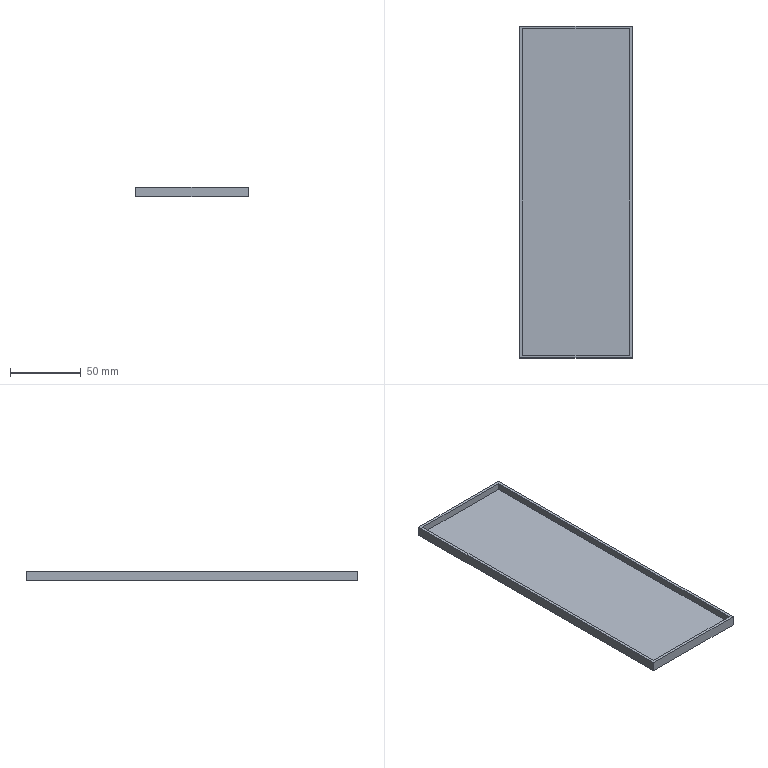Part | NX | features solid 2 | 1 solid | 11 faces | box 79.493 x 234.569 x 7 mm | volume 43494 mm3 | plane 11
STEP:
#1=CARTESIAN_POINT('',(-81.813,268.431,-296.));
#2=VERTEX_POINT('',#1);
#3=CARTESIAN_POINT('',(-161.306,268.431,-296.));
#4=VERTEX_POINT('',#3);
#5=CARTESIAN_POINT('',(-84.813,268.431,-296.));
#6=DIRECTION('',(-1.,0.,0.));
#7=VECTOR('',#6,1000.);
#8=LINE('',#5,#7);
#9=EDGE_CURVE('',#2,#4,#8,.T.);
#10=ORIENTED_EDGE('',*,*,#9,.T.);
#11=CARTESIAN_POINT('',(-161.306,268.431,-303.));
#12=VERTEX_POINT('',#11);
#13=CARTESIAN_POINT('',(-161.306,268.431,-303.));
#14=DIRECTION('',(0.,0.,1.));
#15=VECTOR('',#14,1000.);
#16=LINE('',#13,#15);
#17=EDGE_CURVE('',#12,#4,#16,.T.);
#18=ORIENTED_EDGE('',*,*,#17,.F.);
#19=CARTESIAN_POINT('',(-81.813,268.431,-303.));
#20=VERTEX_POINT('',#19);
#21=CARTESIAN_POINT('',(-84.813,268.431,-303.));
#22=DIRECTION('',(-1.,0.,0.));
#23=VECTOR('',#22,1000.);
#24=LINE('',#21,#23);
#25=EDGE_CURVE('',#20,#12,#24,.T.);
#26=ORIENTED_EDGE('',*,*,#25,.F.);
#27=CARTESIAN_POINT('',(-81.813,268.431,-303.));
#28=DIRECTION('',(0.,0.,1.));
#29=VECTOR('',#28,1000.);
#30=LINE('',#27,#29);
#31=EDGE_CURVE('',#20,#2,#30,.T.);
#32=ORIENTED_EDGE('',*,*,#31,.T.);
#33=EDGE_LOOP('',(#10,#18,#26,#32));
#34=FACE_BOUND('',#33,.T.);
#35=CARTESIAN_POINT('',(-84.813,268.431,-303.));
#36=DIRECTION('',(0.,1.,0.));
#37=DIRECTION('',(0.,0.,1.));
#38=AXIS2_PLACEMENT_3D('',#35,#36,#37);
#39=PLANE('',#38);
#40=ADVANCED_FACE('',(#34),#39,.F.);
#41=CARTESIAN_POINT('',(-161.306,503.,-296.));
#42=VERTEX_POINT('',#41);
#43=CARTESIAN_POINT('',(-161.306,311.431,-296.));
#44=DIRECTION('',(0.,1.,0.));
#45=VECTOR('',#44,1000.);
#46=LINE('',#43,#45);
#47=EDGE_CURVE('',#4,#42,#46,.T.);
#48=ORIENTED_EDGE('',*,*,#47,.T.);
#49=CARTESIAN_POINT('',(-161.306,503.,-303.));
#50=VERTEX_POINT('',#49);
#51=CARTESIAN_POINT('',(-161.306,503.,-303.));
#52=DIRECTION('',(0.,0.,1.));
#53=VECTOR('',#52,1000.);
#54=LINE('',#51,#53);
#55=EDGE_CURVE('',#50,#42,#54,.T.);
#56=ORIENTED_EDGE('',*,*,#55,.F.);
#57=CARTESIAN_POINT('',(-161.306,311.431,-303.));
#58=DIRECTION('',(0.,1.,0.));
#59=VECTOR('',#58,1000.);
#60=LINE('',#57,#59);
#61=EDGE_CURVE('',#12,#50,#60,.T.);
#62=ORIENTED_EDGE('',*,*,#61,.F.);
#63=ORIENTED_EDGE('',*,*,#17,.T.);
#64=EDGE_LOOP('',(#48,#56,#62,#63));
#65=FACE_BOUND('',#64,.T.);
#66=CARTESIAN_POINT('',(-161.306,311.431,-303.));
#67=DIRECTION('',(1.,0.,0.));
#68=DIRECTION('',(0.,0.,-1.));
#69=AXIS2_PLACEMENT_3D('',#66,#67,#68);
#70=PLANE('',#69);
#71=ADVANCED_FACE('',(#65),#70,.F.);
#72=CARTESIAN_POINT('',(-81.813,503.,-296.));
#73=VERTEX_POINT('',#72);
#74=CARTESIAN_POINT('',(-340.,503.,-296.));
#75=DIRECTION('',(1.,0.,0.));
#76=VECTOR('',#75,1000.);
#77=LINE('',#74,#76);
#78=EDGE_CURVE('',#42,#73,#77,.T.);
#79=ORIENTED_EDGE('',*,*,#78,.T.);
#80=CARTESIAN_POINT('',(-81.813,503.,-303.));
#81=VERTEX_POINT('',#80);
#82=CARTESIAN_POINT('',(-81.813,503.,-303.));
#83=DIRECTION('',(0.,0.,1.));
#84=VECTOR('',#83,1000.);
#85=LINE('',#82,#84);
#86=EDGE_CURVE('',#81,#73,#85,.T.);
#87=ORIENTED_EDGE('',*,*,#86,.F.);
#88=CARTESIAN_POINT('',(-340.,503.,-303.));
#89=DIRECTION('',(1.,0.,0.));
#90=VECTOR('',#89,1000.);
#91=LINE('',#88,#90);
#92=EDGE_CURVE('',#50,#81,#91,.T.);
#93=ORIENTED_EDGE('',*,*,#92,.F.);
#94=ORIENTED_EDGE('',*,*,#55,.T.);
#95=EDGE_LOOP('',(#79,#87,#93,#94));
#96=FACE_BOUND('',#95,.T.);
#97=CARTESIAN_POINT('',(-340.,503.,-303.));
#98=DIRECTION('',(0.,-1.,0.));
#99=DIRECTION('',(1.,0.,0.));
#100=AXIS2_PLACEMENT_3D('',#97,#98,#99);
#101=PLANE('',#100);
#102=ADVANCED_FACE('',(#96),#101,.F.);
#103=CARTESIAN_POINT('',(-81.813,500.89,-296.));
#104=DIRECTION('',(0.,-1.,0.));
#105=VECTOR('',#104,1000.);
#106=LINE('',#103,#105);
#107=EDGE_CURVE('',#73,#2,#106,.T.);
#108=ORIENTED_EDGE('',*,*,#107,.T.);
#109=ORIENTED_EDGE('',*,*,#31,.F.);
#110=CARTESIAN_POINT('',(-81.813,500.89,-303.));
#111=DIRECTION('',(0.,-1.,0.));
#112=VECTOR('',#111,1000.);
#113=LINE('',#110,#112);
#114=EDGE_CURVE('',#81,#20,#113,.T.);
#115=ORIENTED_EDGE('',*,*,#114,.F.);
#116=ORIENTED_EDGE('',*,*,#86,.T.);
#117=EDGE_LOOP('',(#108,#109,#115,#116));
#118=FACE_BOUND('',#117,.T.);
#119=CARTESIAN_POINT('',(-81.813,500.89,-303.));
#120=DIRECTION('',(-1.,0.,0.));
#121=DIRECTION('',(0.,0.,1.));
#122=AXIS2_PLACEMENT_3D('',#119,#120,#121);
#123=PLANE('',#122);
#124=ADVANCED_FACE('',(#118),#123,.F.);
#125=ORIENTED_EDGE('',*,*,#25,.T.);
#126=ORIENTED_EDGE('',*,*,#61,.T.);
#127=ORIENTED_EDGE('',*,*,#92,.T.);
#128=ORIENTED_EDGE('',*,*,#114,.T.);
#129=EDGE_LOOP('',(#125,#126,#127,#128));
#130=FACE_BOUND('',#129,.T.);
#131=CARTESIAN_POINT('',(-158.306,311.431,-303.));
#132=DIRECTION('',(0.,0.,-1.));
#133=DIRECTION('',(-1.,0.,0.));
#134=AXIS2_PLACEMENT_3D('',#131,#132,#133);
#135=PLANE('',#134);
#136=ADVANCED_FACE('',(#130),#135,.T.);
#137=CARTESIAN_POINT('',(-83.813,501.,-296.));
#138=VERTEX_POINT('',#137);
#139=CARTESIAN_POINT('',(-83.813,270.431,-296.));
#140=VERTEX_POINT('',#139);
#141=CARTESIAN_POINT('',(-83.813,500.89,-296.));
#142=DIRECTION('',(0.,-1.,0.));
#143=VECTOR('',#142,1000.);
#144=LINE('',#141,#143);
#145=EDGE_CURVE('',#138,#140,#144,.T.);
#146=ORIENTED_EDGE('',*,*,#145,.T.);
#147=CARTESIAN_POINT('',(-159.306,270.431,-296.));
#148=VERTEX_POINT('',#147);
#149=CARTESIAN_POINT('',(-84.813,270.431,-296.));
#150=DIRECTION('',(-1.,0.,0.));
#151=VECTOR('',#150,1000.);
#152=LINE('',#149,#151);
#153=EDGE_CURVE('',#140,#148,#152,.T.);
#154=ORIENTED_EDGE('',*,*,#153,.T.);
#155=CARTESIAN_POINT('',(-159.306,501.,-296.));
#156=VERTEX_POINT('',#155);
#157=CARTESIAN_POINT('',(-159.306,311.431,-296.));
#158=DIRECTION('',(0.,1.,0.));
#159=VECTOR('',#158,1000.);
#160=LINE('',#157,#159);
#161=EDGE_CURVE('',#148,#156,#160,.T.);
#162=ORIENTED_EDGE('',*,*,#161,.T.);
#163=CARTESIAN_POINT('',(-340.,501.,-296.));
#164=DIRECTION('',(1.,0.,0.));
#165=VECTOR('',#164,1000.);
#166=LINE('',#163,#165);
#167=EDGE_CURVE('',#156,#138,#166,.T.);
#168=ORIENTED_EDGE('',*,*,#167,.T.);
#169=EDGE_LOOP('',(#146,#154,#162,#168));
#170=FACE_BOUND('',#169,.T.);
#171=ORIENTED_EDGE('',*,*,#9,.F.);
#172=ORIENTED_EDGE('',*,*,#107,.F.);
#173=ORIENTED_EDGE('',*,*,#78,.F.);
#174=ORIENTED_EDGE('',*,*,#47,.F.);
#175=EDGE_LOOP('',(#171,#172,#173,#174));
#176=FACE_BOUND('',#175,.T.);
#177=CARTESIAN_POINT('',(-158.306,311.431,-296.));
#178=DIRECTION('',(0.,0.,-1.));
#179=DIRECTION('',(-1.,0.,0.));
#180=AXIS2_PLACEMENT_3D('',#177,#178,#179);
#181=PLANE('',#180);
#182=ADVANCED_FACE('',(#170,#176),#181,.F.);
#183=ORIENTED_EDGE('',*,*,#153,.F.);
#184=CARTESIAN_POINT('',(-83.813,270.431,-301.));
#185=VERTEX_POINT('',#184);
#186=CARTESIAN_POINT('',(-83.813,270.431,-303.));
#187=DIRECTION('',(0.,0.,1.));
#188=VECTOR('',#187,1000.);
#189=LINE('',#186,#188);
#190=EDGE_CURVE('',#185,#140,#189,.T.);
#191=ORIENTED_EDGE('',*,*,#190,.F.);
#192=CARTESIAN_POINT('',(-159.306,270.431,-301.));
#193=VERTEX_POINT('',#192);
#194=CARTESIAN_POINT('',(-84.813,270.431,-301.));
#195=DIRECTION('',(-1.,0.,0.));
#196=VECTOR('',#195,1000.);
#197=LINE('',#194,#196);
#198=EDGE_CURVE('',#185,#193,#197,.T.);
#199=ORIENTED_EDGE('',*,*,#198,.T.);
#200=CARTESIAN_POINT('',(-159.306,270.431,-303.));
#201=DIRECTION('',(0.,0.,1.));
#202=VECTOR('',#201,1000.);
#203=LINE('',#200,#202);
#204=EDGE_CURVE('',#193,#148,#203,.T.);
#205=ORIENTED_EDGE('',*,*,#204,.T.);
#206=EDGE_LOOP('',(#183,#191,#199,#205));
#207=FACE_BOUND('',#206,.T.);
#208=CARTESIAN_POINT('',(-84.813,270.431,-303.));
#209=DIRECTION('',(0.,1.,0.));
#210=DIRECTION('',(0.,0.,1.));
#211=AXIS2_PLACEMENT_3D('',#208,#209,#210);
#212=PLANE('',#211);
#213=ADVANCED_FACE('',(#207),#212,.T.);
#214=ORIENTED_EDGE('',*,*,#161,.F.);
#215=ORIENTED_EDGE('',*,*,#204,.F.);
#216=CARTESIAN_POINT('',(-159.306,501.,-301.));
#217=VERTEX_POINT('',#216);
#218=CARTESIAN_POINT('',(-159.306,311.431,-301.));
#219=DIRECTION('',(0.,1.,0.));
#220=VECTOR('',#219,1000.);
#221=LINE('',#218,#220);
#222=EDGE_CURVE('',#193,#217,#221,.T.);
#223=ORIENTED_EDGE('',*,*,#222,.T.);
#224=CARTESIAN_POINT('',(-159.306,501.,-303.));
#225=DIRECTION('',(0.,0.,1.));
#226=VECTOR('',#225,1000.);
#227=LINE('',#224,#226);
#228=EDGE_CURVE('',#217,#156,#227,.T.);
#229=ORIENTED_EDGE('',*,*,#228,.T.);
#230=EDGE_LOOP('',(#214,#215,#223,#229));
#231=FACE_BOUND('',#230,.T.);
#232=CARTESIAN_POINT('',(-159.306,311.431,-303.));
#233=DIRECTION('',(1.,0.,0.));
#234=DIRECTION('',(0.,0.,-1.));
#235=AXIS2_PLACEMENT_3D('',#232,#233,#234);
#236=PLANE('',#235);
#237=ADVANCED_FACE('',(#231),#236,.T.);
#238=ORIENTED_EDGE('',*,*,#167,.F.);
#239=ORIENTED_EDGE('',*,*,#228,.F.);
#240=CARTESIAN_POINT('',(-83.813,501.,-301.));
#241=VERTEX_POINT('',#240);
#242=CARTESIAN_POINT('',(-340.,501.,-301.));
#243=DIRECTION('',(1.,0.,0.));
#244=VECTOR('',#243,1000.);
#245=LINE('',#242,#244);
#246=EDGE_CURVE('',#217,#241,#245,.T.);
#247=ORIENTED_EDGE('',*,*,#246,.T.);
#248=CARTESIAN_POINT('',(-83.813,501.,-303.));
#249=DIRECTION('',(0.,0.,1.));
#250=VECTOR('',#249,1000.);
#251=LINE('',#248,#250);
#252=EDGE_CURVE('',#241,#138,#251,.T.);
#253=ORIENTED_EDGE('',*,*,#252,.T.);
#254=EDGE_LOOP('',(#238,#239,#247,#253));
#255=FACE_BOUND('',#254,.T.);
#256=CARTESIAN_POINT('',(-340.,501.,-303.));
#257=DIRECTION('',(0.,-1.,0.));
#258=DIRECTION('',(1.,0.,0.));
#259=AXIS2_PLACEMENT_3D('',#256,#257,#258);
#260=PLANE('',#259);
#261=ADVANCED_FACE('',(#255),#260,.T.);
#262=ORIENTED_EDGE('',*,*,#145,.F.);
#263=ORIENTED_EDGE('',*,*,#252,.F.);
#264=CARTESIAN_POINT('',(-83.813,500.89,-301.));
#265=DIRECTION('',(0.,-1.,0.));
#266=VECTOR('',#265,1000.);
#267=LINE('',#264,#266);
#268=EDGE_CURVE('',#241,#185,#267,.T.);
#269=ORIENTED_EDGE('',*,*,#268,.T.);
#270=ORIENTED_EDGE('',*,*,#190,.T.);
#271=EDGE_LOOP('',(#262,#263,#269,#270));
#272=FACE_BOUND('',#271,.T.);
#273=CARTESIAN_POINT('',(-83.813,500.89,-303.));
#274=DIRECTION('',(-1.,0.,0.));
#275=DIRECTION('',(0.,0.,1.));
#276=AXIS2_PLACEMENT_3D('',#273,#274,#275);
#277=PLANE('',#276);
#278=ADVANCED_FACE('',(#272),#277,.T.);
#279=ORIENTED_EDGE('',*,*,#198,.F.);
#280=ORIENTED_EDGE('',*,*,#268,.F.);
#281=ORIENTED_EDGE('',*,*,#246,.F.);
#282=ORIENTED_EDGE('',*,*,#222,.F.);
#283=EDGE_LOOP('',(#279,#280,#281,#282));
#284=FACE_BOUND('',#283,.T.);
#285=CARTESIAN_POINT('',(-158.306,311.431,-301.));
#286=DIRECTION('',(0.,0.,-1.));
#287=DIRECTION('',(-1.,0.,0.));
#288=AXIS2_PLACEMENT_3D('',#285,#286,#287);
#289=PLANE('',#288);
#290=ADVANCED_FACE('',(#284),#289,.F.);
#291=CLOSED_SHELL('',(#40,#71,#102,#124,#136,#182,#213,#237,#261,#278,#290));
#292=MANIFOLD_SOLID_BREP('',#291);
#293=(LENGTH_UNIT()NAMED_UNIT(*)SI_UNIT(.MILLI.,.METRE.));
#294=UNCERTAINTY_MEASURE_WITH_UNIT(LENGTH_MEASURE(0.00001),#293,'','');
#295=(NAMED_UNIT(*)PLANE_ANGLE_UNIT()SI_UNIT($,.RADIAN.));
#296=(NAMED_UNIT(*)SI_UNIT($,.STERADIAN.)SOLID_ANGLE_UNIT());
#297=(GEOMETRIC_REPRESENTATION_CONTEXT(3)GLOBAL_UNCERTAINTY_ASSIGNED_CONTEXT((#294))GLOBAL_UNIT_ASSIGNED_CONTEXT((#293,#295,#296))REPRESENTATION_CONTEXT('',''));
#298=ADVANCED_BREP_SHAPE_REPRESENTATION('',(#292),#297);